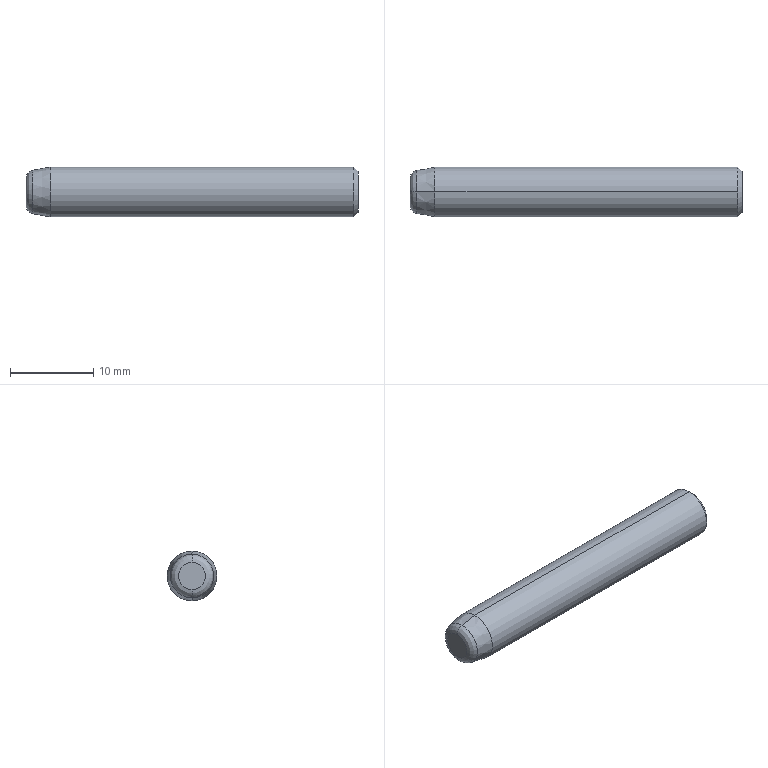Part | STEP file | Pino guia - PNG-0640 - M4 | 1 solid | 19 faces | box 40 x 6 x 6 mm | volume 979.582 mm3 | cone 8 | cylinder 6 | plane 3 | torus 2 | commonest cylinder face diameters 3.3 x2 4 x2 6 x2
STEP:
#1=CARTESIAN_POINT('',(0.,0.,0.));
#2=DIRECTION('',(0.,0.,1.));
#3=DIRECTION('',(1.,0.,0.));
#4=AXIS2_PLACEMENT_3D('',#1,#2,#3);
#5=CARTESIAN_POINT('',(-39.174,0.,2.617));
#6=VERTEX_POINT('',#5);
#7=CARTESIAN_POINT('',(-39.174,0.,-2.617));
#8=VERTEX_POINT('',#7);
#9=CARTESIAN_POINT('',(-39.174,0.,0.));
#10=DIRECTION('',(-1.,0.,0.));
#11=DIRECTION('',(0.,0.,1.));
#12=AXIS2_PLACEMENT_3D('',#9,#10,#11);
#13=CIRCLE('',#12,2.617);
#14=CARTESIAN_POINT('',(-39.,0.,0.));
#15=DIRECTION('',(-1.,0.,0.));
#16=DIRECTION('',(0.,0.,1.));
#17=AXIS2_PLACEMENT_3D('',#14,#15,#16);
#18=TOROIDAL_SURFACE('',#17,1.632,1.);
#19=CARTESIAN_POINT('',(0.,0.1745));
#20=DIRECTION('',(1.,0.));
#21=VECTOR('',#20,1.);
#22=LINE('',#19,#21);
#23=(GEOMETRIC_REPRESENTATION_CONTEXT(2)PARAMETRIC_REPRESENTATION_CONTEXT()REPRESENTATION_CONTEXT('',''));
#24=DEFINITIONAL_REPRESENTATION('',(#22),#23);
#25=PCURVE('',#18,#24);
#26=CARTESIAN_POINT('',(-37.,0.,0.));
#27=DIRECTION('',(1.,0.,0.));
#28=DIRECTION('',(0.,0.,-1.));
#29=AXIS2_PLACEMENT_3D('',#26,#27,#28);
#30=CONICAL_SURFACE('',#29,3.,0.1745);
#31=CARTESIAN_POINT('',(3.142,-2.174));
#32=DIRECTION('',(-1.,0.));
#33=VECTOR('',#32,1.);
#34=LINE('',#31,#33);
#35=(GEOMETRIC_REPRESENTATION_CONTEXT(2)PARAMETRIC_REPRESENTATION_CONTEXT()REPRESENTATION_CONTEXT('',''));
#36=DEFINITIONAL_REPRESENTATION('',(#34),#35);
#37=PCURVE('',#30,#36);
#38=SURFACE_CURVE('',#13,(#25,#37),.PCURVE_S1.);
#39=EDGE_CURVE('',#6,#8,#38,.T.);
#40=ORIENTED_EDGE('',*,*,#39,.T.);
#41=CARTESIAN_POINT('',(-40.,0.,-1.632));
#42=VERTEX_POINT('',#41);
#43=CARTESIAN_POINT('',(-39.,0.,-1.632));
#44=DIRECTION('',(0.,1.,0.));
#45=DIRECTION('',(0.,0.,1.));
#46=AXIS2_PLACEMENT_3D('',#43,#44,#45);
#47=CIRCLE('',#46,1.);
#48=CARTESIAN_POINT('',(3.142,-3.142));
#49=DIRECTION('',(0.,1.));
#50=VECTOR('',#49,1.);
#51=LINE('',#48,#50);
#52=(GEOMETRIC_REPRESENTATION_CONTEXT(2)PARAMETRIC_REPRESENTATION_CONTEXT()REPRESENTATION_CONTEXT('',''));
#53=DEFINITIONAL_REPRESENTATION('',(#51),#52);
#54=PCURVE('',#18,#53);
#55=CARTESIAN_POINT('',(-39.,0.,0.));
#56=DIRECTION('',(-1.,0.,0.));
#57=DIRECTION('',(0.,0.,1.));
#58=AXIS2_PLACEMENT_3D('',#55,#56,#57);
#59=TOROIDAL_SURFACE('',#58,1.632,1.);
#60=CARTESIAN_POINT('',(3.142,-3.142));
#61=DIRECTION('',(0.,1.));
#62=VECTOR('',#61,1.);
#63=LINE('',#60,#62);
#64=(GEOMETRIC_REPRESENTATION_CONTEXT(2)PARAMETRIC_REPRESENTATION_CONTEXT()REPRESENTATION_CONTEXT('',''));
#65=DEFINITIONAL_REPRESENTATION('',(#63),#64);
#66=PCURVE('',#59,#65);
#67=SURFACE_CURVE('',#47,(#54,#66),.PCURVE_S1.);
#68=EDGE_CURVE('',#8,#42,#67,.T.);
#69=ORIENTED_EDGE('',*,*,#68,.T.);
#70=CARTESIAN_POINT('',(-40.,0.,1.632));
#71=VERTEX_POINT('',#70);
#72=CARTESIAN_POINT('',(-40.,0.,0.));
#73=DIRECTION('',(-1.,0.,0.));
#74=DIRECTION('',(0.,0.,1.));
#75=AXIS2_PLACEMENT_3D('',#72,#73,#74);
#76=CIRCLE('',#75,1.632);
#77=CARTESIAN_POINT('',(0.,1.571));
#78=DIRECTION('',(1.,0.));
#79=VECTOR('',#78,1.);
#80=LINE('',#77,#79);
#81=(GEOMETRIC_REPRESENTATION_CONTEXT(2)PARAMETRIC_REPRESENTATION_CONTEXT()REPRESENTATION_CONTEXT('',''));
#82=DEFINITIONAL_REPRESENTATION('',(#80),#81);
#83=PCURVE('',#18,#82);
#84=CARTESIAN_POINT('',(-40.,0.,-1.632));
#85=DIRECTION('',(1.,0.,0.));
#86=DIRECTION('',(0.,0.,-1.));
#87=AXIS2_PLACEMENT_3D('',#84,#85,#86);
#88=PLANE('',#87);
#89=CARTESIAN_POINT('',(-3.264,0.));
#90=CARTESIAN_POINT('',(-3.264,2.827));
#91=CARTESIAN_POINT('',(-0.816,1.413));
#92=CARTESIAN_POINT('',(1.632,0.));
#93=CARTESIAN_POINT('',(-0.816,-1.413));
#94=CARTESIAN_POINT('',(-3.264,-2.827));
#95=CARTESIAN_POINT('',(-3.264,0.));
#96=(BOUNDED_CURVE()B_SPLINE_CURVE(2,(#89,#90,#91,#92,#93,#94,#95),.UNSPECIFIED.,.T.,.F.)B_SPLINE_CURVE_WITH_KNOTS((1,2,2,2,2,1),(-2.094,0.,2.094,4.189,6.283,8.378),.UNSPECIFIED.)CURVE()GEOMETRIC_REPRESENTATION_ITEM()RATIONAL_B_SPLINE_CURVE((1.,0.5,1.,0.5,1.,0.5,1.))REPRESENTATION_ITEM(''));
#97=(GEOMETRIC_REPRESENTATION_CONTEXT(2)PARAMETRIC_REPRESENTATION_CONTEXT()REPRESENTATION_CONTEXT('',''));
#98=DEFINITIONAL_REPRESENTATION('',(#96),#97);
#99=PCURVE('',#88,#98);
#100=SURFACE_CURVE('',#76,(#83,#99),.PCURVE_S1.);
#101=EDGE_CURVE('',#71,#42,#100,.T.);
#102=ORIENTED_EDGE('',*,*,#101,.F.);
#103=CARTESIAN_POINT('',(-39.,0.,1.632));
#104=DIRECTION('',(0.,-1.,0.));
#105=DIRECTION('',(0.,0.,-1.));
#106=AXIS2_PLACEMENT_3D('',#103,#104,#105);
#107=CIRCLE('',#106,1.);
#108=CARTESIAN_POINT('',(0.,-3.142));
#109=DIRECTION('',(0.,1.));
#110=VECTOR('',#109,1.);
#111=LINE('',#108,#110);
#112=(GEOMETRIC_REPRESENTATION_CONTEXT(2)PARAMETRIC_REPRESENTATION_CONTEXT()REPRESENTATION_CONTEXT('',''));
#113=DEFINITIONAL_REPRESENTATION('',(#111),#112);
#114=PCURVE('',#18,#113);
#115=CARTESIAN_POINT('',(6.283,-3.142));
#116=DIRECTION('',(0.,1.));
#117=VECTOR('',#116,1.);
#118=LINE('',#115,#117);
#119=(GEOMETRIC_REPRESENTATION_CONTEXT(2)PARAMETRIC_REPRESENTATION_CONTEXT()REPRESENTATION_CONTEXT('',''));
#120=DEFINITIONAL_REPRESENTATION('',(#118),#119);
#121=PCURVE('',#59,#120);
#122=SURFACE_CURVE('',#107,(#114,#121),.PCURVE_S1.);
#123=EDGE_CURVE('',#6,#71,#122,.T.);
#124=ORIENTED_EDGE('',*,*,#123,.F.);
#125=EDGE_LOOP('',(#40,#69,#102,#124));
#126=FACE_BOUND('',#125,.T.);
#127=ADVANCED_FACE('',(#126),#18,.T.);
#128=ORIENTED_EDGE('',*,*,#39,.F.);
#129=CARTESIAN_POINT('',(-37.,0.,3.));
#130=VERTEX_POINT('',#129);
#131=CARTESIAN_POINT('',(-37.,0.,3.));
#132=DIRECTION('',(0.9848,0.,0.1736));
#133=VECTOR('',#132,1.);
#134=LINE('',#131,#133);
#135=CARTESIAN_POINT('',(3.142,0.));
#136=DIRECTION('',(0.,1.));
#137=VECTOR('',#136,1.);
#138=LINE('',#135,#137);
#139=(GEOMETRIC_REPRESENTATION_CONTEXT(2)PARAMETRIC_REPRESENTATION_CONTEXT()REPRESENTATION_CONTEXT('',''));
#140=DEFINITIONAL_REPRESENTATION('',(#138),#139);
#141=PCURVE('',#30,#140);
#142=CARTESIAN_POINT('',(-37.,0.,0.));
#143=DIRECTION('',(1.,0.,0.));
#144=DIRECTION('',(0.,0.,-1.));
#145=AXIS2_PLACEMENT_3D('',#142,#143,#144);
#146=CONICAL_SURFACE('',#145,3.,0.1745);
#147=CARTESIAN_POINT('',(3.142,0.));
#148=DIRECTION('',(0.,1.));
#149=VECTOR('',#148,1.);
#150=LINE('',#147,#149);
#151=(GEOMETRIC_REPRESENTATION_CONTEXT(2)PARAMETRIC_REPRESENTATION_CONTEXT()REPRESENTATION_CONTEXT('',''));
#152=DEFINITIONAL_REPRESENTATION('',(#150),#151);
#153=PCURVE('',#146,#152);
#154=SURFACE_CURVE('',#134,(#141,#153),.PCURVE_S1.);
#155=EDGE_CURVE('',#6,#130,#154,.T.);
#156=ORIENTED_EDGE('',*,*,#155,.T.);
#157=CARTESIAN_POINT('',(-37.,0.,-3.));
#158=VERTEX_POINT('',#157);
#159=CARTESIAN_POINT('',(-37.,0.,0.));
#160=DIRECTION('',(-1.,0.,0.));
#161=DIRECTION('',(0.,0.,1.));
#162=AXIS2_PLACEMENT_3D('',#159,#160,#161);
#163=CIRCLE('',#162,3.);
#164=CARTESIAN_POINT('',(3.142,0.));
#165=DIRECTION('',(-1.,0.));
#166=VECTOR('',#165,1.);
#167=LINE('',#164,#166);
#168=(GEOMETRIC_REPRESENTATION_CONTEXT(2)PARAMETRIC_REPRESENTATION_CONTEXT()REPRESENTATION_CONTEXT('',''));
#169=DEFINITIONAL_REPRESENTATION('',(#167),#168);
#170=PCURVE('',#30,#169);
#171=CARTESIAN_POINT('',(-5.343,0.,0.));
#172=DIRECTION('',(-1.,0.,0.));
#173=DIRECTION('',(0.,0.,1.));
#174=AXIS2_PLACEMENT_3D('',#171,#172,#173);
#175=CYLINDRICAL_SURFACE('',#174,3.);
#176=CARTESIAN_POINT('',(0.,31.657));
#177=DIRECTION('',(1.,0.));
#178=VECTOR('',#177,1.);
#179=LINE('',#176,#178);
#180=(GEOMETRIC_REPRESENTATION_CONTEXT(2)PARAMETRIC_REPRESENTATION_CONTEXT()REPRESENTATION_CONTEXT('',''));
#181=DEFINITIONAL_REPRESENTATION('',(#179),#180);
#182=PCURVE('',#175,#181);
#183=SURFACE_CURVE('',#163,(#170,#182),.PCURVE_S1.);
#184=EDGE_CURVE('',#130,#158,#183,.T.);
#185=ORIENTED_EDGE('',*,*,#184,.T.);
#186=CARTESIAN_POINT('',(-37.,0.,-3.));
#187=DIRECTION('',(0.9848,0.,-0.1736));
#188=VECTOR('',#187,1.);
#189=LINE('',#186,#188);
#190=CARTESIAN_POINT('',(0.,0.));
#191=DIRECTION('',(0.,1.));
#192=VECTOR('',#191,1.);
#193=LINE('',#190,#192);
#194=(GEOMETRIC_REPRESENTATION_CONTEXT(2)PARAMETRIC_REPRESENTATION_CONTEXT()REPRESENTATION_CONTEXT('',''));
#195=DEFINITIONAL_REPRESENTATION('',(#193),#194);
#196=PCURVE('',#30,#195);
#197=CARTESIAN_POINT('',(6.283,0.));
#198=DIRECTION('',(0.,1.));
#199=VECTOR('',#198,1.);
#200=LINE('',#197,#199);
#201=(GEOMETRIC_REPRESENTATION_CONTEXT(2)PARAMETRIC_REPRESENTATION_CONTEXT()REPRESENTATION_CONTEXT('',''));
#202=DEFINITIONAL_REPRESENTATION('',(#200),#201);
#203=PCURVE('',#146,#202);
#204=SURFACE_CURVE('',#189,(#196,#203),.PCURVE_S1.);
#205=EDGE_CURVE('',#8,#158,#204,.T.);
#206=ORIENTED_EDGE('',*,*,#205,.F.);
#207=EDGE_LOOP('',(#128,#156,#185,#206));
#208=FACE_BOUND('',#207,.T.);
#209=ADVANCED_FACE('',(#208),#30,.T.);
#210=CARTESIAN_POINT('',(-0.025,0.,-2.));
#211=VERTEX_POINT('',#210);
#212=CARTESIAN_POINT('',(0.,0.,-2.025));
#213=VERTEX_POINT('',#212);
#214=CARTESIAN_POINT('',(0.,0.,-2.025));
#215=DIRECTION('',(0.7071,0.,-0.7071));
#216=VECTOR('',#215,1.);
#217=LINE('',#214,#216);
#218=CARTESIAN_POINT('',(0.,0.,0.));
#219=DIRECTION('',(1.,0.,0.));
#220=DIRECTION('',(0.,0.,-1.));
#221=AXIS2_PLACEMENT_3D('',#218,#219,#220);
#222=CONICAL_SURFACE('',#221,2.025,0.7854);
#223=CARTESIAN_POINT('',(6.283,0.));
#224=DIRECTION('',(0.,1.));
#225=VECTOR('',#224,1.);
#226=LINE('',#223,#225);
#227=(GEOMETRIC_REPRESENTATION_CONTEXT(2)PARAMETRIC_REPRESENTATION_CONTEXT()REPRESENTATION_CONTEXT('',''));
#228=DEFINITIONAL_REPRESENTATION('',(#226),#227);
#229=PCURVE('',#222,#228);
#230=CARTESIAN_POINT('',(0.,0.,0.));
#231=DIRECTION('',(1.,0.,0.));
#232=DIRECTION('',(0.,0.,-1.));
#233=AXIS2_PLACEMENT_3D('',#230,#231,#232);
#234=CONICAL_SURFACE('',#233,2.025,0.7854);
#235=CARTESIAN_POINT('',(0.,0.));
#236=DIRECTION('',(0.,1.));
#237=VECTOR('',#236,1.);
#238=LINE('',#235,#237);
#239=(GEOMETRIC_REPRESENTATION_CONTEXT(2)PARAMETRIC_REPRESENTATION_CONTEXT()REPRESENTATION_CONTEXT('',''));
#240=DEFINITIONAL_REPRESENTATION('',(#238),#239);
#241=PCURVE('',#234,#240);
#242=SURFACE_CURVE('',#217,(#229,#241),.PCURVE_S1.);
#243=EDGE_CURVE('',#211,#213,#242,.T.);
#244=ORIENTED_EDGE('',*,*,#243,.T.);
#245=CARTESIAN_POINT('',(0.,0.,2.025));
#246=VERTEX_POINT('',#245);
#247=CARTESIAN_POINT('',(0.,0.,0.));
#248=DIRECTION('',(1.,0.,0.));
#249=DIRECTION('',(0.,0.,-1.));
#250=AXIS2_PLACEMENT_3D('',#247,#248,#249);
#251=CIRCLE('',#250,2.025);
#252=CARTESIAN_POINT('',(0.,0.));
#253=DIRECTION('',(1.,0.));
#254=VECTOR('',#253,1.);
#255=LINE('',#252,#254);
#256=(GEOMETRIC_REPRESENTATION_CONTEXT(2)PARAMETRIC_REPRESENTATION_CONTEXT()REPRESENTATION_CONTEXT('',''));
#257=DEFINITIONAL_REPRESENTATION('',(#255),#256);
#258=PCURVE('',#222,#257);
#259=CARTESIAN_POINT('',(0.,2.5,0.));
#260=DIRECTION('',(-1.,0.,0.));
#261=DIRECTION('',(0.,0.,1.));
#262=AXIS2_PLACEMENT_3D('',#259,#260,#261);
#263=PLANE('',#262);
#264=CARTESIAN_POINT('',(-2.025,-2.5));
#265=CARTESIAN_POINT('',(-2.025,1.007));
#266=CARTESIAN_POINT('',(1.012,-0.7463));
#267=CARTESIAN_POINT('',(4.05,-2.5));
#268=CARTESIAN_POINT('',(1.012,-4.254));
#269=CARTESIAN_POINT('',(-2.025,-6.007));
#270=CARTESIAN_POINT('',(-2.025,-2.5));
#271=(BOUNDED_CURVE()B_SPLINE_CURVE(2,(#264,#265,#266,#267,#268,#269,#270),.UNSPECIFIED.,.T.,.F.)B_SPLINE_CURVE_WITH_KNOTS((1,2,2,2,2,1),(-2.094,0.,2.094,4.189,6.283,8.378),.UNSPECIFIED.)CURVE()GEOMETRIC_REPRESENTATION_ITEM()RATIONAL_B_SPLINE_CURVE((1.,0.5,1.,0.5,1.,0.5,1.))REPRESENTATION_ITEM(''));
#272=(GEOMETRIC_REPRESENTATION_CONTEXT(2)PARAMETRIC_REPRESENTATION_CONTEXT()REPRESENTATION_CONTEXT('',''));
#273=DEFINITIONAL_REPRESENTATION('',(#271),#272);
#274=PCURVE('',#263,#273);
#275=SURFACE_CURVE('',#251,(#258,#274),.PCURVE_S1.);
#276=EDGE_CURVE('',#246,#213,#275,.T.);
#277=ORIENTED_EDGE('',*,*,#276,.F.);
#278=CARTESIAN_POINT('',(-0.025,0.,2.));
#279=VERTEX_POINT('',#278);
#280=CARTESIAN_POINT('',(0.,0.,2.025));
#281=DIRECTION('',(0.7071,0.,0.7071));
#282=VECTOR('',#281,1.);
#283=LINE('',#280,#282);
#284=CARTESIAN_POINT('',(3.142,0.));
#285=DIRECTION('',(0.,1.));
#286=VECTOR('',#285,1.);
#287=LINE('',#284,#286);
#288=(GEOMETRIC_REPRESENTATION_CONTEXT(2)PARAMETRIC_REPRESENTATION_CONTEXT()REPRESENTATION_CONTEXT('',''));
#289=DEFINITIONAL_REPRESENTATION('',(#287),#288);
#290=PCURVE('',#222,#289);
#291=CARTESIAN_POINT('',(3.142,0.));
#292=DIRECTION('',(0.,1.));
#293=VECTOR('',#292,1.);
#294=LINE('',#291,#293);
#295=(GEOMETRIC_REPRESENTATION_CONTEXT(2)PARAMETRIC_REPRESENTATION_CONTEXT()REPRESENTATION_CONTEXT('',''));
#296=DEFINITIONAL_REPRESENTATION('',(#294),#295);
#297=PCURVE('',#234,#296);
#298=SURFACE_CURVE('',#283,(#290,#297),.PCURVE_S1.);
#299=EDGE_CURVE('',#279,#246,#298,.T.);
#300=ORIENTED_EDGE('',*,*,#299,.F.);
#301=CARTESIAN_POINT('',(-0.025,0.,0.));
#302=DIRECTION('',(1.,0.,0.));
#303=DIRECTION('',(0.,0.,-1.));
#304=AXIS2_PLACEMENT_3D('',#301,#302,#303);
#305=CIRCLE('',#304,2.);
#306=CARTESIAN_POINT('',(0.,-0.025));
#307=DIRECTION('',(1.,0.));
#308=VECTOR('',#307,1.);
#309=LINE('',#306,#308);
#310=(GEOMETRIC_REPRESENTATION_CONTEXT(2)PARAMETRIC_REPRESENTATION_CONTEXT()REPRESENTATION_CONTEXT('',''));
#311=DEFINITIONAL_REPRESENTATION('',(#309),#310);
#312=PCURVE('',#222,#311);
#313=CARTESIAN_POINT('',(0.,0.,0.));
#314=DIRECTION('',(1.,0.,0.));
#315=DIRECTION('',(0.,0.,-1.));
#316=AXIS2_PLACEMENT_3D('',#313,#314,#315);
#317=CYLINDRICAL_SURFACE('',#316,2.);
#318=CARTESIAN_POINT('',(0.,-0.025));
#319=DIRECTION('',(1.,0.));
#320=VECTOR('',#319,1.);
#321=LINE('',#318,#320);
#322=(GEOMETRIC_REPRESENTATION_CONTEXT(2)PARAMETRIC_REPRESENTATION_CONTEXT()REPRESENTATION_CONTEXT('',''));
#323=DEFINITIONAL_REPRESENTATION('',(#321),#322);
#324=PCURVE('',#317,#323);
#325=SURFACE_CURVE('',#305,(#312,#324),.PCURVE_S1.);
#326=EDGE_CURVE('',#279,#211,#325,.T.);
#327=ORIENTED_EDGE('',*,*,#326,.T.);
#328=EDGE_LOOP('',(#244,#277,#300,#327));
#329=FACE_BOUND('',#328,.F.);
#330=ADVANCED_FACE('',(#329),#222,.F.);
#331=CARTESIAN_POINT('',(-9.,0.,-2.));
#332=VERTEX_POINT('',#331);
#333=CARTESIAN_POINT('',(0.,0.,-2.));
#334=DIRECTION('',(1.,0.,0.));
#335=VECTOR('',#334,1.);
#336=LINE('',#333,#335);
#337=CARTESIAN_POINT('',(6.283,0.));
#338=DIRECTION('',(0.,1.));
#339=VECTOR('',#338,1.);
#340=LINE('',#337,#339);
#341=(GEOMETRIC_REPRESENTATION_CONTEXT(2)PARAMETRIC_REPRESENTATION_CONTEXT()REPRESENTATION_CONTEXT('',''));
#342=DEFINITIONAL_REPRESENTATION('',(#340),#341);
#343=PCURVE('',#317,#342);
#344=CARTESIAN_POINT('',(0.,0.,0.));
#345=DIRECTION('',(1.,0.,0.));
#346=DIRECTION('',(0.,0.,-1.));
#347=AXIS2_PLACEMENT_3D('',#344,#345,#346);
#348=CYLINDRICAL_SURFACE('',#347,2.);
#349=CARTESIAN_POINT('',(0.,0.));
#350=DIRECTION('',(0.,1.));
#351=VECTOR('',#350,1.);
#352=LINE('',#349,#351);
#353=(GEOMETRIC_REPRESENTATION_CONTEXT(2)PARAMETRIC_REPRESENTATION_CONTEXT()REPRESENTATION_CONTEXT('',''));
#354=DEFINITIONAL_REPRESENTATION('',(#352),#353);
#355=PCURVE('',#348,#354);
#356=SURFACE_CURVE('',#336,(#343,#355),.PCURVE_S1.);
#357=EDGE_CURVE('',#332,#211,#356,.T.);
#358=ORIENTED_EDGE('',*,*,#357,.T.);
#359=ORIENTED_EDGE('',*,*,#326,.F.);
#360=CARTESIAN_POINT('',(-9.,0.,2.));
#361=VERTEX_POINT('',#360);
#362=CARTESIAN_POINT('',(0.,0.,2.));
#363=DIRECTION('',(1.,0.,0.));
#364=VECTOR('',#363,1.);
#365=LINE('',#362,#364);
#366=CARTESIAN_POINT('',(3.142,0.));
#367=DIRECTION('',(0.,1.));
#368=VECTOR('',#367,1.);
#369=LINE('',#366,#368);
#370=(GEOMETRIC_REPRESENTATION_CONTEXT(2)PARAMETRIC_REPRESENTATION_CONTEXT()REPRESENTATION_CONTEXT('',''));
#371=DEFINITIONAL_REPRESENTATION('',(#369),#370);
#372=PCURVE('',#317,#371);
#373=CARTESIAN_POINT('',(3.142,0.));
#374=DIRECTION('',(0.,1.));
#375=VECTOR('',#374,1.);
#376=LINE('',#373,#375);
#377=(GEOMETRIC_REPRESENTATION_CONTEXT(2)PARAMETRIC_REPRESENTATION_CONTEXT()REPRESENTATION_CONTEXT('',''));
#378=DEFINITIONAL_REPRESENTATION('',(#376),#377);
#379=PCURVE('',#348,#378);
#380=SURFACE_CURVE('',#365,(#372,#379),.PCURVE_S1.);
#381=EDGE_CURVE('',#361,#279,#380,.T.);
#382=ORIENTED_EDGE('',*,*,#381,.F.);
#383=CARTESIAN_POINT('',(-9.,0.,0.));
#384=DIRECTION('',(1.,0.,0.));
#385=DIRECTION('',(0.,0.,-1.));
#386=AXIS2_PLACEMENT_3D('',#383,#384,#385);
#387=CIRCLE('',#386,2.);
#388=CARTESIAN_POINT('',(0.,-9.));
#389=DIRECTION('',(1.,0.));
#390=VECTOR('',#389,1.);
#391=LINE('',#388,#390);
#392=(GEOMETRIC_REPRESENTATION_CONTEXT(2)PARAMETRIC_REPRESENTATION_CONTEXT()REPRESENTATION_CONTEXT('',''));
#393=DEFINITIONAL_REPRESENTATION('',(#391),#392);
#394=PCURVE('',#317,#393);
#395=CARTESIAN_POINT('',(-9.,1.65,0.));
#396=DIRECTION('',(-1.,0.,0.));
#397=DIRECTION('',(0.,0.,1.));
#398=AXIS2_PLACEMENT_3D('',#395,#396,#397);
#399=PLANE('',#398);
#400=CARTESIAN_POINT('',(-2.,-1.65));
#401=CARTESIAN_POINT('',(-2.,1.814));
#402=CARTESIAN_POINT('',(1.,0.08205));
#403=CARTESIAN_POINT('',(4.,-1.65));
#404=CARTESIAN_POINT('',(1.,-3.382));
#405=CARTESIAN_POINT('',(-2.,-5.114));
#406=CARTESIAN_POINT('',(-2.,-1.65));
#407=(BOUNDED_CURVE()B_SPLINE_CURVE(2,(#400,#401,#402,#403,#404,#405,#406),.UNSPECIFIED.,.T.,.F.)B_SPLINE_CURVE_WITH_KNOTS((1,2,2,2,2,1),(-2.094,0.,2.094,4.189,6.283,8.378),.UNSPECIFIED.)CURVE()GEOMETRIC_REPRESENTATION_ITEM()RATIONAL_B_SPLINE_CURVE((1.,0.5,1.,0.5,1.,0.5,1.))REPRESENTATION_ITEM(''));
#408=(GEOMETRIC_REPRESENTATION_CONTEXT(2)PARAMETRIC_REPRESENTATION_CONTEXT()REPRESENTATION_CONTEXT('',''));
#409=DEFINITIONAL_REPRESENTATION('',(#407),#408);
#410=PCURVE('',#399,#409);
#411=SURFACE_CURVE('',#387,(#394,#410),.PCURVE_S1.);
#412=EDGE_CURVE('',#361,#332,#411,.T.);
#413=ORIENTED_EDGE('',*,*,#412,.T.);
#414=EDGE_LOOP('',(#358,#359,#382,#413));
#415=FACE_BOUND('',#414,.F.);
#416=ADVANCED_FACE('',(#415),#317,.F.);
#417=CARTESIAN_POINT('',(-11.,0.,-1.65));
#418=VERTEX_POINT('',#417);
#419=CARTESIAN_POINT('',(-9.,0.,-1.65));
#420=VERTEX_POINT('',#419);
#421=CARTESIAN_POINT('',(0.,0.,-1.65));
#422=DIRECTION('',(1.,0.,0.));
#423=VECTOR('',#422,1.);
#424=LINE('',#421,#423);
#425=CARTESIAN_POINT('',(0.,0.,0.));
#426=DIRECTION('',(1.,0.,0.));
#427=DIRECTION('',(0.,0.,-1.));
#428=AXIS2_PLACEMENT_3D('',#425,#426,#427);
#429=CYLINDRICAL_SURFACE('',#428,1.65);
#430=CARTESIAN_POINT('',(6.283,0.));
#431=DIRECTION('',(0.,1.));
#432=VECTOR('',#431,1.);
#433=LINE('',#430,#432);
#434=(GEOMETRIC_REPRESENTATION_CONTEXT(2)PARAMETRIC_REPRESENTATION_CONTEXT()REPRESENTATION_CONTEXT('',''));
#435=DEFINITIONAL_REPRESENTATION('',(#433),#434);
#436=PCURVE('',#429,#435);
#437=CARTESIAN_POINT('',(0.,0.,0.));
#438=DIRECTION('',(1.,0.,0.));
#439=DIRECTION('',(0.,0.,-1.));
#440=AXIS2_PLACEMENT_3D('',#437,#438,#439);
#441=CYLINDRICAL_SURFACE('',#440,1.65);
#442=CARTESIAN_POINT('',(0.,0.));
#443=DIRECTION('',(0.,1.));
#444=VECTOR('',#443,1.);
#445=LINE('',#442,#444);
#446=(GEOMETRIC_REPRESENTATION_CONTEXT(2)PARAMETRIC_REPRESENTATION_CONTEXT()REPRESENTATION_CONTEXT('',''));
#447=DEFINITIONAL_REPRESENTATION('',(#445),#446);
#448=PCURVE('',#441,#447);
#449=SURFACE_CURVE('',#424,(#436,#448),.PCURVE_S1.);
#450=EDGE_CURVE('',#418,#420,#449,.T.);
#451=ORIENTED_EDGE('',*,*,#450,.T.);
#452=CARTESIAN_POINT('',(-9.,0.,1.65));
#453=VERTEX_POINT('',#452);
#454=CARTESIAN_POINT('',(-9.,0.,0.));
#455=DIRECTION('',(1.,0.,0.));
#456=DIRECTION('',(0.,0.,-1.));
#457=AXIS2_PLACEMENT_3D('',#454,#455,#456);
#458=CIRCLE('',#457,1.65);
#459=CARTESIAN_POINT('',(0.,-9.));
#460=DIRECTION('',(1.,0.));
#461=VECTOR('',#460,1.);
#462=LINE('',#459,#461);
#463=(GEOMETRIC_REPRESENTATION_CONTEXT(2)PARAMETRIC_REPRESENTATION_CONTEXT()REPRESENTATION_CONTEXT('',''));
#464=DEFINITIONAL_REPRESENTATION('',(#462),#463);
#465=PCURVE('',#429,#464);
#466=CARTESIAN_POINT('',(-1.65,-1.65));
#467=CARTESIAN_POINT('',(-1.65,1.208));
#468=CARTESIAN_POINT('',(0.825,-0.2211));
#469=CARTESIAN_POINT('',(3.3,-1.65));
#470=CARTESIAN_POINT('',(0.825,-3.079));
#471=CARTESIAN_POINT('',(-1.65,-4.508));
#472=CARTESIAN_POINT('',(-1.65,-1.65));
#473=(BOUNDED_CURVE()B_SPLINE_CURVE(2,(#466,#467,#468,#469,#470,#471,#472),.UNSPECIFIED.,.T.,.F.)B_SPLINE_CURVE_WITH_KNOTS((1,2,2,2,2,1),(-2.094,0.,2.094,4.189,6.283,8.378),.UNSPECIFIED.)CURVE()GEOMETRIC_REPRESENTATION_ITEM()RATIONAL_B_SPLINE_CURVE((1.,0.5,1.,0.5,1.,0.5,1.))REPRESENTATION_ITEM(''));
#474=(GEOMETRIC_REPRESENTATION_CONTEXT(2)PARAMETRIC_REPRESENTATION_CONTEXT()REPRESENTATION_CONTEXT('',''));
#475=DEFINITIONAL_REPRESENTATION('',(#473),#474);
#476=PCURVE('',#399,#475);
#477=SURFACE_CURVE('',#458,(#465,#476),.PCURVE_S1.);
#478=EDGE_CURVE('',#453,#420,#477,.T.);
#479=ORIENTED_EDGE('',*,*,#478,.F.);
#480=CARTESIAN_POINT('',(-11.,0.,1.65));
#481=VERTEX_POINT('',#480);
#482=CARTESIAN_POINT('',(0.,0.,1.65));
#483=DIRECTION('',(1.,0.,0.));
#484=VECTOR('',#483,1.);
#485=LINE('',#482,#484);
#486=CARTESIAN_POINT('',(3.142,0.));
#487=DIRECTION('',(0.,1.));
#488=VECTOR('',#487,1.);
#489=LINE('',#486,#488);
#490=(GEOMETRIC_REPRESENTATION_CONTEXT(2)PARAMETRIC_REPRESENTATION_CONTEXT()REPRESENTATION_CONTEXT('',''));
#491=DEFINITIONAL_REPRESENTATION('',(#489),#490);
#492=PCURVE('',#429,#491);
#493=CARTESIAN_POINT('',(3.142,0.));
#494=DIRECTION('',(0.,1.));
#495=VECTOR('',#494,1.);
#496=LINE('',#493,#495);
#497=(GEOMETRIC_REPRESENTATION_CONTEXT(2)PARAMETRIC_REPRESENTATION_CONTEXT()REPRESENTATION_CONTEXT('',''));
#498=DEFINITIONAL_REPRESENTATION('',(#496),#497);
#499=PCURVE('',#441,#498);
#500=SURFACE_CURVE('',#485,(#492,#499),.PCURVE_S1.);
#501=EDGE_CURVE('',#481,#453,#500,.T.);
#502=ORIENTED_EDGE('',*,*,#501,.F.);
#503=CARTESIAN_POINT('',(-11.,0.,0.));
#504=DIRECTION('',(1.,0.,0.));
#505=DIRECTION('',(0.,0.,-1.));
#506=AXIS2_PLACEMENT_3D('',#503,#504,#505);
#507=CIRCLE('',#506,1.65);
#508=CARTESIAN_POINT('',(0.,-11.));
#509=DIRECTION('',(1.,0.));
#510=VECTOR('',#509,1.);
#511=LINE('',#508,#510);
#512=(GEOMETRIC_REPRESENTATION_CONTEXT(2)PARAMETRIC_REPRESENTATION_CONTEXT()REPRESENTATION_CONTEXT('',''));
#513=DEFINITIONAL_REPRESENTATION('',(#511),#512);
#514=PCURVE('',#429,#513);
#515=CARTESIAN_POINT('',(-11.,0.,0.));
#516=DIRECTION('',(1.,0.,0.));
#517=DIRECTION('',(0.,0.,-1.));
#518=AXIS2_PLACEMENT_3D('',#515,#516,#517);
#519=CONICAL_SURFACE('',#518,1.65,1.03);
#520=CARTESIAN_POINT('',(0.,0.));
#521=DIRECTION('',(1.,0.));
#522=VECTOR('',#521,1.);
#523=LINE('',#520,#522);
#524=(GEOMETRIC_REPRESENTATION_CONTEXT(2)PARAMETRIC_REPRESENTATION_CONTEXT()REPRESENTATION_CONTEXT('',''));
#525=DEFINITIONAL_REPRESENTATION('',(#523),#524);
#526=PCURVE('',#519,#525);
#527=SURFACE_CURVE('',#507,(#514,#526),.PCURVE_S1.);
#528=EDGE_CURVE('',#481,#418,#527,.T.);
#529=ORIENTED_EDGE('',*,*,#528,.T.);
#530=EDGE_LOOP('',(#451,#479,#502,#529));
#531=FACE_BOUND('',#530,.F.);
#532=ADVANCED_FACE('',(#531),#429,.F.);
#533=ORIENTED_EDGE('',*,*,#528,.F.);
#534=CARTESIAN_POINT('',(-11.991,0.,0.));
#535=VERTEX_POINT('',#534);
#536=CARTESIAN_POINT('',(-11.,0.,1.65));
#537=DIRECTION('',(0.515,0.,0.8572));
#538=VECTOR('',#537,1.);
#539=LINE('',#536,#538);
#540=CARTESIAN_POINT('',(3.142,0.));
#541=DIRECTION('',(0.,1.));
#542=VECTOR('',#541,1.);
#543=LINE('',#540,#542);
#544=(GEOMETRIC_REPRESENTATION_CONTEXT(2)PARAMETRIC_REPRESENTATION_CONTEXT()REPRESENTATION_CONTEXT('',''));
#545=DEFINITIONAL_REPRESENTATION('',(#543),#544);
#546=PCURVE('',#519,#545);
#547=CARTESIAN_POINT('',(-11.,0.,0.));
#548=DIRECTION('',(1.,0.,0.));
#549=DIRECTION('',(0.,0.,-1.));
#550=AXIS2_PLACEMENT_3D('',#547,#548,#549);
#551=CONICAL_SURFACE('',#550,1.65,1.03);
#552=CARTESIAN_POINT('',(3.142,0.));
#553=DIRECTION('',(0.,1.));
#554=VECTOR('',#553,1.);
#555=LINE('',#552,#554);
#556=(GEOMETRIC_REPRESENTATION_CONTEXT(2)PARAMETRIC_REPRESENTATION_CONTEXT()REPRESENTATION_CONTEXT('',''));
#557=DEFINITIONAL_REPRESENTATION('',(#555),#556);
#558=PCURVE('',#551,#557);
#559=SURFACE_CURVE('',#539,(#546,#558),.PCURVE_S1.);
#560=EDGE_CURVE('',#535,#481,#559,.T.);
#561=ORIENTED_EDGE('',*,*,#560,.F.);
#562=CARTESIAN_POINT('',(-11.,0.,-1.65));
#563=DIRECTION('',(0.515,0.,-0.8572));
#564=VECTOR('',#563,1.);
#565=LINE('',#562,#564);
#566=CARTESIAN_POINT('',(6.283,0.));
#567=DIRECTION('',(0.,1.));
#568=VECTOR('',#567,1.);
#569=LINE('',#566,#568);
#570=(GEOMETRIC_REPRESENTATION_CONTEXT(2)PARAMETRIC_REPRESENTATION_CONTEXT()REPRESENTATION_CONTEXT('',''));
#571=DEFINITIONAL_REPRESENTATION('',(#569),#570);
#572=PCURVE('',#519,#571);
#573=CARTESIAN_POINT('',(0.,0.));
#574=DIRECTION('',(0.,1.));
#575=VECTOR('',#574,1.);
#576=LINE('',#573,#575);
#577=(GEOMETRIC_REPRESENTATION_CONTEXT(2)PARAMETRIC_REPRESENTATION_CONTEXT()REPRESENTATION_CONTEXT('',''));
#578=DEFINITIONAL_REPRESENTATION('',(#576),#577);
#579=PCURVE('',#551,#578);
#580=SURFACE_CURVE('',#565,(#572,#579),.PCURVE_S1.);
#581=EDGE_CURVE('',#535,#418,#580,.T.);
#582=ORIENTED_EDGE('',*,*,#581,.T.);
#583=EDGE_LOOP('',(#533,#561,#582));
#584=FACE_BOUND('',#583,.F.);
#585=ADVANCED_FACE('',(#584),#519,.F.);
#586=CARTESIAN_POINT('',(-0.5,0.,3.));
#587=VERTEX_POINT('',#586);
#588=CARTESIAN_POINT('',(-0.5,0.,-3.));
#589=VERTEX_POINT('',#588);
#590=CARTESIAN_POINT('',(-0.5,0.,0.));
#591=DIRECTION('',(-1.,0.,0.));
#592=DIRECTION('',(0.,0.,1.));
#593=AXIS2_PLACEMENT_3D('',#590,#591,#592);
#594=CIRCLE('',#593,3.);
#595=CARTESIAN_POINT('',(0.,-4.843));
#596=DIRECTION('',(1.,0.));
#597=VECTOR('',#596,1.);
#598=LINE('',#595,#597);
#599=(GEOMETRIC_REPRESENTATION_CONTEXT(2)PARAMETRIC_REPRESENTATION_CONTEXT()REPRESENTATION_CONTEXT('',''));
#600=DEFINITIONAL_REPRESENTATION('',(#598),#599);
#601=PCURVE('',#175,#600);
#602=CARTESIAN_POINT('',(0.,0.,0.));
#603=DIRECTION('',(-1.,0.,0.));
#604=DIRECTION('',(0.,0.,1.));
#605=AXIS2_PLACEMENT_3D('',#602,#603,#604);
#606=CONICAL_SURFACE('',#605,2.5,0.7854);
#607=CARTESIAN_POINT('',(0.,0.5));
#608=DIRECTION('',(1.,0.));
#609=VECTOR('',#608,1.);
#610=LINE('',#607,#609);
#611=(GEOMETRIC_REPRESENTATION_CONTEXT(2)PARAMETRIC_REPRESENTATION_CONTEXT()REPRESENTATION_CONTEXT('',''));
#612=DEFINITIONAL_REPRESENTATION('',(#610),#611);
#613=PCURVE('',#606,#612);
#614=SURFACE_CURVE('',#594,(#601,#613),.PCURVE_S1.);
#615=EDGE_CURVE('',#587,#589,#614,.T.);
#616=ORIENTED_EDGE('',*,*,#615,.T.);
#617=CARTESIAN_POINT('',(-5.343,0.,-3.));
#618=DIRECTION('',(-1.,0.,0.));
#619=VECTOR('',#618,1.);
#620=LINE('',#617,#619);
#621=CARTESIAN_POINT('',(3.142,0.));
#622=DIRECTION('',(0.,1.));
#623=VECTOR('',#622,1.);
#624=LINE('',#621,#623);
#625=(GEOMETRIC_REPRESENTATION_CONTEXT(2)PARAMETRIC_REPRESENTATION_CONTEXT()REPRESENTATION_CONTEXT('',''));
#626=DEFINITIONAL_REPRESENTATION('',(#624),#625);
#627=PCURVE('',#175,#626);
#628=CARTESIAN_POINT('',(-5.343,0.,0.));
#629=DIRECTION('',(-1.,0.,0.));
#630=DIRECTION('',(0.,0.,1.));
#631=AXIS2_PLACEMENT_3D('',#628,#629,#630);
#632=CYLINDRICAL_SURFACE('',#631,3.);
#633=CARTESIAN_POINT('',(3.142,0.));
#634=DIRECTION('',(0.,1.));
#635=VECTOR('',#634,1.);
#636=LINE('',#633,#635);
#637=(GEOMETRIC_REPRESENTATION_CONTEXT(2)PARAMETRIC_REPRESENTATION_CONTEXT()REPRESENTATION_CONTEXT('',''));
#638=DEFINITIONAL_REPRESENTATION('',(#636),#637);
#639=PCURVE('',#632,#638);
#640=SURFACE_CURVE('',#620,(#627,#639),.PCURVE_S1.);
#641=EDGE_CURVE('',#589,#158,#640,.T.);
#642=ORIENTED_EDGE('',*,*,#641,.T.);
#643=ORIENTED_EDGE('',*,*,#184,.F.);
#644=CARTESIAN_POINT('',(-5.343,0.,3.));
#645=DIRECTION('',(-1.,0.,0.));
#646=VECTOR('',#645,1.);
#647=LINE('',#644,#646);
#648=CARTESIAN_POINT('',(0.,0.));
#649=DIRECTION('',(0.,1.));
#650=VECTOR('',#649,1.);
#651=LINE('',#648,#650);
#652=(GEOMETRIC_REPRESENTATION_CONTEXT(2)PARAMETRIC_REPRESENTATION_CONTEXT()REPRESENTATION_CONTEXT('',''));
#653=DEFINITIONAL_REPRESENTATION('',(#651),#652);
#654=PCURVE('',#175,#653);
#655=CARTESIAN_POINT('',(6.283,0.));
#656=DIRECTION('',(0.,1.));
#657=VECTOR('',#656,1.);
#658=LINE('',#655,#657);
#659=(GEOMETRIC_REPRESENTATION_CONTEXT(2)PARAMETRIC_REPRESENTATION_CONTEXT()REPRESENTATION_CONTEXT('',''));
#660=DEFINITIONAL_REPRESENTATION('',(#658),#659);
#661=PCURVE('',#632,#660);
#662=SURFACE_CURVE('',#647,(#654,#661),.PCURVE_S1.);
#663=EDGE_CURVE('',#587,#130,#662,.T.);
#664=ORIENTED_EDGE('',*,*,#663,.F.);
#665=EDGE_LOOP('',(#616,#642,#643,#664));
#666=FACE_BOUND('',#665,.T.);
#667=ADVANCED_FACE('',(#666),#175,.T.);
#668=CARTESIAN_POINT('',(0.,0.,2.5));
#669=VERTEX_POINT('',#668);
#670=CARTESIAN_POINT('',(0.,0.,-2.5));
#671=VERTEX_POINT('',#670);
#672=CARTESIAN_POINT('',(0.,0.,0.));
#673=DIRECTION('',(-1.,0.,0.));
#674=DIRECTION('',(0.,0.,1.));
#675=AXIS2_PLACEMENT_3D('',#672,#673,#674);
#676=CIRCLE('',#675,2.5);
#677=CARTESIAN_POINT('',(0.,0.));
#678=DIRECTION('',(1.,0.));
#679=VECTOR('',#678,1.);
#680=LINE('',#677,#679);
#681=(GEOMETRIC_REPRESENTATION_CONTEXT(2)PARAMETRIC_REPRESENTATION_CONTEXT()REPRESENTATION_CONTEXT('',''));
#682=DEFINITIONAL_REPRESENTATION('',(#680),#681);
#683=PCURVE('',#606,#682);
#684=CARTESIAN_POINT('',(0.,-2.5));
#685=DIRECTION('',(1.,0.));
#686=AXIS2_PLACEMENT_2D('',#684,#685);
#687=CIRCLE('',#686,2.5);
#688=(GEOMETRIC_REPRESENTATION_CONTEXT(2)PARAMETRIC_REPRESENTATION_CONTEXT()REPRESENTATION_CONTEXT('',''));
#689=DEFINITIONAL_REPRESENTATION('',(#687),#688);
#690=PCURVE('',#263,#689);
#691=SURFACE_CURVE('',#676,(#683,#690),.PCURVE_S1.);
#692=EDGE_CURVE('',#669,#671,#691,.T.);
#693=ORIENTED_EDGE('',*,*,#692,.T.);
#694=CARTESIAN_POINT('',(0.,0.,-2.5));
#695=DIRECTION('',(-0.7071,0.,-0.7071));
#696=VECTOR('',#695,1.);
#697=LINE('',#694,#696);
#698=CARTESIAN_POINT('',(3.142,0.));
#699=DIRECTION('',(0.,1.));
#700=VECTOR('',#699,1.);
#701=LINE('',#698,#700);
#702=(GEOMETRIC_REPRESENTATION_CONTEXT(2)PARAMETRIC_REPRESENTATION_CONTEXT()REPRESENTATION_CONTEXT('',''));
#703=DEFINITIONAL_REPRESENTATION('',(#701),#702);
#704=PCURVE('',#606,#703);
#705=CARTESIAN_POINT('',(0.,0.,0.));
#706=DIRECTION('',(-1.,0.,0.));
#707=DIRECTION('',(0.,0.,1.));
#708=AXIS2_PLACEMENT_3D('',#705,#706,#707);
#709=CONICAL_SURFACE('',#708,2.5,0.7854);
#710=CARTESIAN_POINT('',(3.142,0.));
#711=DIRECTION('',(0.,1.));
#712=VECTOR('',#711,1.);
#713=LINE('',#710,#712);
#714=(GEOMETRIC_REPRESENTATION_CONTEXT(2)PARAMETRIC_REPRESENTATION_CONTEXT()REPRESENTATION_CONTEXT('',''));
#715=DEFINITIONAL_REPRESENTATION('',(#713),#714);
#716=PCURVE('',#709,#715);
#717=SURFACE_CURVE('',#697,(#704,#716),.PCURVE_S1.);
#718=EDGE_CURVE('',#671,#589,#717,.T.);
#719=ORIENTED_EDGE('',*,*,#718,.T.);
#720=ORIENTED_EDGE('',*,*,#615,.F.);
#721=CARTESIAN_POINT('',(0.,0.,2.5));
#722=DIRECTION('',(-0.7071,0.,0.7071));
#723=VECTOR('',#722,1.);
#724=LINE('',#721,#723);
#725=CARTESIAN_POINT('',(0.,0.));
#726=DIRECTION('',(0.,1.));
#727=VECTOR('',#726,1.);
#728=LINE('',#725,#727);
#729=(GEOMETRIC_REPRESENTATION_CONTEXT(2)PARAMETRIC_REPRESENTATION_CONTEXT()REPRESENTATION_CONTEXT('',''));
#730=DEFINITIONAL_REPRESENTATION('',(#728),#729);
#731=PCURVE('',#606,#730);
#732=CARTESIAN_POINT('',(6.283,0.));
#733=DIRECTION('',(0.,1.));
#734=VECTOR('',#733,1.);
#735=LINE('',#732,#734);
#736=(GEOMETRIC_REPRESENTATION_CONTEXT(2)PARAMETRIC_REPRESENTATION_CONTEXT()REPRESENTATION_CONTEXT('',''));
#737=DEFINITIONAL_REPRESENTATION('',(#735),#736);
#738=PCURVE('',#709,#737);
#739=SURFACE_CURVE('',#724,(#731,#738),.PCURVE_S1.);
#740=EDGE_CURVE('',#669,#587,#739,.T.);
#741=ORIENTED_EDGE('',*,*,#740,.F.);
#742=EDGE_LOOP('',(#693,#719,#720,#741));
#743=FACE_BOUND('',#742,.T.);
#744=ADVANCED_FACE('',(#743),#606,.T.);
#745=CARTESIAN_POINT('',(0.,0.,0.));
#746=DIRECTION('',(1.,0.,0.));
#747=DIRECTION('',(0.,0.,-1.));
#748=AXIS2_PLACEMENT_3D('',#745,#746,#747);
#749=CIRCLE('',#748,2.025);
#750=CARTESIAN_POINT('',(-2.025,-2.5));
#751=CARTESIAN_POINT('',(-2.025,1.007));
#752=CARTESIAN_POINT('',(1.012,-0.7463));
#753=CARTESIAN_POINT('',(4.05,-2.5));
#754=CARTESIAN_POINT('',(1.012,-4.254));
#755=CARTESIAN_POINT('',(-2.025,-6.007));
#756=CARTESIAN_POINT('',(-2.025,-2.5));
#757=(BOUNDED_CURVE()B_SPLINE_CURVE(2,(#750,#751,#752,#753,#754,#755,#756),.UNSPECIFIED.,.T.,.F.)B_SPLINE_CURVE_WITH_KNOTS((1,2,2,2,2,1),(-2.094,0.,2.094,4.189,6.283,8.378),.UNSPECIFIED.)CURVE()GEOMETRIC_REPRESENTATION_ITEM()RATIONAL_B_SPLINE_CURVE((1.,0.5,1.,0.5,1.,0.5,1.))REPRESENTATION_ITEM(''));
#758=(GEOMETRIC_REPRESENTATION_CONTEXT(2)PARAMETRIC_REPRESENTATION_CONTEXT()REPRESENTATION_CONTEXT('',''));
#759=DEFINITIONAL_REPRESENTATION('',(#757),#758);
#760=PCURVE('',#263,#759);
#761=CARTESIAN_POINT('',(0.,0.));
#762=DIRECTION('',(1.,0.));
#763=VECTOR('',#762,1.);
#764=LINE('',#761,#763);
#765=(GEOMETRIC_REPRESENTATION_CONTEXT(2)PARAMETRIC_REPRESENTATION_CONTEXT()REPRESENTATION_CONTEXT('',''));
#766=DEFINITIONAL_REPRESENTATION('',(#764),#765);
#767=PCURVE('',#234,#766);
#768=SURFACE_CURVE('',#749,(#760,#767),.PCURVE_S1.);
#769=EDGE_CURVE('',#213,#246,#768,.T.);
#770=ORIENTED_EDGE('',*,*,#769,.F.);
#771=ORIENTED_EDGE('',*,*,#276,.F.);
#772=EDGE_LOOP('',(#770,#771));
#773=FACE_BOUND('',#772,.T.);
#774=ORIENTED_EDGE('',*,*,#692,.F.);
#775=CARTESIAN_POINT('',(0.,0.,0.));
#776=DIRECTION('',(-1.,0.,0.));
#777=DIRECTION('',(0.,0.,1.));
#778=AXIS2_PLACEMENT_3D('',#775,#776,#777);
#779=CIRCLE('',#778,2.5);
#780=CARTESIAN_POINT('',(0.,-2.5));
#781=DIRECTION('',(1.,0.));
#782=AXIS2_PLACEMENT_2D('',#780,#781);
#783=CIRCLE('',#782,2.5);
#784=(GEOMETRIC_REPRESENTATION_CONTEXT(2)PARAMETRIC_REPRESENTATION_CONTEXT()REPRESENTATION_CONTEXT('',''));
#785=DEFINITIONAL_REPRESENTATION('',(#783),#784);
#786=PCURVE('',#263,#785);
#787=CARTESIAN_POINT('',(0.,0.));
#788=DIRECTION('',(1.,0.));
#789=VECTOR('',#788,1.);
#790=LINE('',#787,#789);
#791=(GEOMETRIC_REPRESENTATION_CONTEXT(2)PARAMETRIC_REPRESENTATION_CONTEXT()REPRESENTATION_CONTEXT('',''));
#792=DEFINITIONAL_REPRESENTATION('',(#790),#791);
#793=PCURVE('',#709,#792);
#794=SURFACE_CURVE('',#779,(#786,#793),.PCURVE_S1.);
#795=EDGE_CURVE('',#671,#669,#794,.T.);
#796=ORIENTED_EDGE('',*,*,#795,.F.);
#797=EDGE_LOOP('',(#774,#796));
#798=FACE_BOUND('',#797,.T.);
#799=ADVANCED_FACE('',(#773,#798),#263,.F.);
#800=ORIENTED_EDGE('',*,*,#718,.F.);
#801=ORIENTED_EDGE('',*,*,#795,.T.);
#802=ORIENTED_EDGE('',*,*,#740,.T.);
#803=CARTESIAN_POINT('',(-0.5,0.,0.));
#804=DIRECTION('',(-1.,0.,0.));
#805=DIRECTION('',(0.,0.,1.));
#806=AXIS2_PLACEMENT_3D('',#803,#804,#805);
#807=CIRCLE('',#806,3.);
#808=CARTESIAN_POINT('',(0.,0.5));
#809=DIRECTION('',(1.,0.));
#810=VECTOR('',#809,1.);
#811=LINE('',#808,#810);
#812=(GEOMETRIC_REPRESENTATION_CONTEXT(2)PARAMETRIC_REPRESENTATION_CONTEXT()REPRESENTATION_CONTEXT('',''));
#813=DEFINITIONAL_REPRESENTATION('',(#811),#812);
#814=PCURVE('',#709,#813);
#815=CARTESIAN_POINT('',(0.,-4.843));
#816=DIRECTION('',(1.,0.));
#817=VECTOR('',#816,1.);
#818=LINE('',#815,#817);
#819=(GEOMETRIC_REPRESENTATION_CONTEXT(2)PARAMETRIC_REPRESENTATION_CONTEXT()REPRESENTATION_CONTEXT('',''));
#820=DEFINITIONAL_REPRESENTATION('',(#818),#819);
#821=PCURVE('',#632,#820);
#822=SURFACE_CURVE('',#807,(#814,#821),.PCURVE_S1.);
#823=EDGE_CURVE('',#589,#587,#822,.T.);
#824=ORIENTED_EDGE('',*,*,#823,.F.);
#825=EDGE_LOOP('',(#800,#801,#802,#824));
#826=FACE_BOUND('',#825,.T.);
#827=ADVANCED_FACE('',(#826),#709,.T.);
#828=ORIENTED_EDGE('',*,*,#641,.F.);
#829=ORIENTED_EDGE('',*,*,#823,.T.);
#830=ORIENTED_EDGE('',*,*,#663,.T.);
#831=CARTESIAN_POINT('',(-37.,0.,0.));
#832=DIRECTION('',(-1.,0.,0.));
#833=DIRECTION('',(0.,0.,1.));
#834=AXIS2_PLACEMENT_3D('',#831,#832,#833);
#835=CIRCLE('',#834,3.);
#836=CARTESIAN_POINT('',(0.,31.657));
#837=DIRECTION('',(1.,0.));
#838=VECTOR('',#837,1.);
#839=LINE('',#836,#838);
#840=(GEOMETRIC_REPRESENTATION_CONTEXT(2)PARAMETRIC_REPRESENTATION_CONTEXT()REPRESENTATION_CONTEXT('',''));
#841=DEFINITIONAL_REPRESENTATION('',(#839),#840);
#842=PCURVE('',#632,#841);
#843=CARTESIAN_POINT('',(9.425,0.));
#844=DIRECTION('',(-1.,0.));
#845=VECTOR('',#844,1.);
#846=LINE('',#843,#845);
#847=(GEOMETRIC_REPRESENTATION_CONTEXT(2)PARAMETRIC_REPRESENTATION_CONTEXT()REPRESENTATION_CONTEXT('',''));
#848=DEFINITIONAL_REPRESENTATION('',(#846),#847);
#849=PCURVE('',#146,#848);
#850=SURFACE_CURVE('',#835,(#842,#849),.PCURVE_S1.);
#851=EDGE_CURVE('',#158,#130,#850,.T.);
#852=ORIENTED_EDGE('',*,*,#851,.F.);
#853=EDGE_LOOP('',(#828,#829,#830,#852));
#854=FACE_BOUND('',#853,.T.);
#855=ADVANCED_FACE('',(#854),#632,.T.);
#856=CARTESIAN_POINT('',(-11.,0.,0.));
#857=DIRECTION('',(1.,0.,0.));
#858=DIRECTION('',(0.,0.,-1.));
#859=AXIS2_PLACEMENT_3D('',#856,#857,#858);
#860=CIRCLE('',#859,1.65);
#861=CARTESIAN_POINT('',(0.,0.));
#862=DIRECTION('',(1.,0.));
#863=VECTOR('',#862,1.);
#864=LINE('',#861,#863);
#865=(GEOMETRIC_REPRESENTATION_CONTEXT(2)PARAMETRIC_REPRESENTATION_CONTEXT()REPRESENTATION_CONTEXT('',''));
#866=DEFINITIONAL_REPRESENTATION('',(#864),#865);
#867=PCURVE('',#551,#866);
#868=CARTESIAN_POINT('',(0.,-11.));
#869=DIRECTION('',(1.,0.));
#870=VECTOR('',#869,1.);
#871=LINE('',#868,#870);
#872=(GEOMETRIC_REPRESENTATION_CONTEXT(2)PARAMETRIC_REPRESENTATION_CONTEXT()REPRESENTATION_CONTEXT('',''));
#873=DEFINITIONAL_REPRESENTATION('',(#871),#872);
#874=PCURVE('',#441,#873);
#875=SURFACE_CURVE('',#860,(#867,#874),.PCURVE_S1.);
#876=EDGE_CURVE('',#418,#481,#875,.T.);
#877=ORIENTED_EDGE('',*,*,#876,.F.);
#878=ORIENTED_EDGE('',*,*,#581,.F.);
#879=ORIENTED_EDGE('',*,*,#560,.T.);
#880=EDGE_LOOP('',(#877,#878,#879));
#881=FACE_BOUND('',#880,.F.);
#882=ADVANCED_FACE('',(#881),#551,.F.);
#883=CARTESIAN_POINT('',(-9.,0.,0.));
#884=DIRECTION('',(1.,0.,0.));
#885=DIRECTION('',(0.,0.,-1.));
#886=AXIS2_PLACEMENT_3D('',#883,#884,#885);
#887=CIRCLE('',#886,1.65);
#888=CARTESIAN_POINT('',(0.,-9.));
#889=DIRECTION('',(1.,0.));
#890=VECTOR('',#889,1.);
#891=LINE('',#888,#890);
#892=(GEOMETRIC_REPRESENTATION_CONTEXT(2)PARAMETRIC_REPRESENTATION_CONTEXT()REPRESENTATION_CONTEXT('',''));
#893=DEFINITIONAL_REPRESENTATION('',(#891),#892);
#894=PCURVE('',#441,#893);
#895=CARTESIAN_POINT('',(-1.65,-1.65));
#896=CARTESIAN_POINT('',(-1.65,1.208));
#897=CARTESIAN_POINT('',(0.825,-0.2211));
#898=CARTESIAN_POINT('',(3.3,-1.65));
#899=CARTESIAN_POINT('',(0.825,-3.079));
#900=CARTESIAN_POINT('',(-1.65,-4.508));
#901=CARTESIAN_POINT('',(-1.65,-1.65));
#902=(BOUNDED_CURVE()B_SPLINE_CURVE(2,(#895,#896,#897,#898,#899,#900,#901),.UNSPECIFIED.,.T.,.F.)B_SPLINE_CURVE_WITH_KNOTS((1,2,2,2,2,1),(-2.094,0.,2.094,4.189,6.283,8.378),.UNSPECIFIED.)CURVE()GEOMETRIC_REPRESENTATION_ITEM()RATIONAL_B_SPLINE_CURVE((1.,0.5,1.,0.5,1.,0.5,1.))REPRESENTATION_ITEM(''));
#903=(GEOMETRIC_REPRESENTATION_CONTEXT(2)PARAMETRIC_REPRESENTATION_CONTEXT()REPRESENTATION_CONTEXT('',''));
#904=DEFINITIONAL_REPRESENTATION('',(#902),#903);
#905=PCURVE('',#399,#904);
#906=SURFACE_CURVE('',#887,(#894,#905),.PCURVE_S1.);
#907=EDGE_CURVE('',#420,#453,#906,.T.);
#908=ORIENTED_EDGE('',*,*,#907,.F.);
#909=ORIENTED_EDGE('',*,*,#450,.F.);
#910=ORIENTED_EDGE('',*,*,#876,.T.);
#911=ORIENTED_EDGE('',*,*,#501,.T.);
#912=EDGE_LOOP('',(#908,#909,#910,#911));
#913=FACE_BOUND('',#912,.F.);
#914=ADVANCED_FACE('',(#913),#441,.F.);
#915=ORIENTED_EDGE('',*,*,#907,.F.);
#916=ORIENTED_EDGE('',*,*,#478,.F.);
#917=EDGE_LOOP('',(#915,#916));
#918=FACE_BOUND('',#917,.T.);
#919=CARTESIAN_POINT('',(-9.,0.,0.));
#920=DIRECTION('',(1.,0.,0.));
#921=DIRECTION('',(0.,0.,-1.));
#922=AXIS2_PLACEMENT_3D('',#919,#920,#921);
#923=CIRCLE('',#922,2.);
#924=CARTESIAN_POINT('',(-2.,-1.65));
#925=CARTESIAN_POINT('',(-2.,1.814));
#926=CARTESIAN_POINT('',(1.,0.08205));
#927=CARTESIAN_POINT('',(4.,-1.65));
#928=CARTESIAN_POINT('',(1.,-3.382));
#929=CARTESIAN_POINT('',(-2.,-5.114));
#930=CARTESIAN_POINT('',(-2.,-1.65));
#931=(BOUNDED_CURVE()B_SPLINE_CURVE(2,(#924,#925,#926,#927,#928,#929,#930),.UNSPECIFIED.,.T.,.F.)B_SPLINE_CURVE_WITH_KNOTS((1,2,2,2,2,1),(-2.094,0.,2.094,4.189,6.283,8.378),.UNSPECIFIED.)CURVE()GEOMETRIC_REPRESENTATION_ITEM()RATIONAL_B_SPLINE_CURVE((1.,0.5,1.,0.5,1.,0.5,1.))REPRESENTATION_ITEM(''));
#932=(GEOMETRIC_REPRESENTATION_CONTEXT(2)PARAMETRIC_REPRESENTATION_CONTEXT()REPRESENTATION_CONTEXT('',''));
#933=DEFINITIONAL_REPRESENTATION('',(#931),#932);
#934=PCURVE('',#399,#933);
#935=CARTESIAN_POINT('',(0.,-9.));
#936=DIRECTION('',(1.,0.));
#937=VECTOR('',#936,1.);
#938=LINE('',#935,#937);
#939=(GEOMETRIC_REPRESENTATION_CONTEXT(2)PARAMETRIC_REPRESENTATION_CONTEXT()REPRESENTATION_CONTEXT('',''));
#940=DEFINITIONAL_REPRESENTATION('',(#938),#939);
#941=PCURVE('',#348,#940);
#942=SURFACE_CURVE('',#923,(#934,#941),.PCURVE_S1.);
#943=EDGE_CURVE('',#332,#361,#942,.T.);
#944=ORIENTED_EDGE('',*,*,#943,.T.);
#945=ORIENTED_EDGE('',*,*,#412,.T.);
#946=EDGE_LOOP('',(#944,#945));
#947=FACE_BOUND('',#946,.T.);
#948=ADVANCED_FACE('',(#918,#947),#399,.F.);
#949=CARTESIAN_POINT('',(-0.025,0.,0.));
#950=DIRECTION('',(1.,0.,0.));
#951=DIRECTION('',(0.,0.,-1.));
#952=AXIS2_PLACEMENT_3D('',#949,#950,#951);
#953=CIRCLE('',#952,2.);
#954=CARTESIAN_POINT('',(0.,-0.025));
#955=DIRECTION('',(1.,0.));
#956=VECTOR('',#955,1.);
#957=LINE('',#954,#956);
#958=(GEOMETRIC_REPRESENTATION_CONTEXT(2)PARAMETRIC_REPRESENTATION_CONTEXT()REPRESENTATION_CONTEXT('',''));
#959=DEFINITIONAL_REPRESENTATION('',(#957),#958);
#960=PCURVE('',#348,#959);
#961=CARTESIAN_POINT('',(0.,-0.025));
#962=DIRECTION('',(1.,0.));
#963=VECTOR('',#962,1.);
#964=LINE('',#961,#963);
#965=(GEOMETRIC_REPRESENTATION_CONTEXT(2)PARAMETRIC_REPRESENTATION_CONTEXT()REPRESENTATION_CONTEXT('',''));
#966=DEFINITIONAL_REPRESENTATION('',(#964),#965);
#967=PCURVE('',#234,#966);
#968=SURFACE_CURVE('',#953,(#960,#967),.PCURVE_S1.);
#969=EDGE_CURVE('',#211,#279,#968,.T.);
#970=ORIENTED_EDGE('',*,*,#969,.F.);
#971=ORIENTED_EDGE('',*,*,#357,.F.);
#972=ORIENTED_EDGE('',*,*,#943,.T.);
#973=ORIENTED_EDGE('',*,*,#381,.T.);
#974=EDGE_LOOP('',(#970,#971,#972,#973));
#975=FACE_BOUND('',#974,.F.);
#976=ADVANCED_FACE('',(#975),#348,.F.);
#977=ORIENTED_EDGE('',*,*,#769,.F.);
#978=ORIENTED_EDGE('',*,*,#243,.F.);
#979=ORIENTED_EDGE('',*,*,#969,.T.);
#980=ORIENTED_EDGE('',*,*,#299,.T.);
#981=EDGE_LOOP('',(#977,#978,#979,#980));
#982=FACE_BOUND('',#981,.F.);
#983=ADVANCED_FACE('',(#982),#234,.F.);
#984=ORIENTED_EDGE('',*,*,#155,.F.);
#985=CARTESIAN_POINT('',(-39.174,0.,0.));
#986=DIRECTION('',(-1.,0.,0.));
#987=DIRECTION('',(0.,0.,1.));
#988=AXIS2_PLACEMENT_3D('',#985,#986,#987);
#989=CIRCLE('',#988,2.617);
#990=CARTESIAN_POINT('',(9.425,-2.174));
#991=DIRECTION('',(-1.,0.));
#992=VECTOR('',#991,1.);
#993=LINE('',#990,#992);
#994=(GEOMETRIC_REPRESENTATION_CONTEXT(2)PARAMETRIC_REPRESENTATION_CONTEXT()REPRESENTATION_CONTEXT('',''));
#995=DEFINITIONAL_REPRESENTATION('',(#993),#994);
#996=PCURVE('',#146,#995);
#997=CARTESIAN_POINT('',(0.,0.1745));
#998=DIRECTION('',(1.,0.));
#999=VECTOR('',#998,1.);
#1000=LINE('',#997,#999);
#1001=(GEOMETRIC_REPRESENTATION_CONTEXT(2)PARAMETRIC_REPRESENTATION_CONTEXT()REPRESENTATION_CONTEXT('',''));
#1002=DEFINITIONAL_REPRESENTATION('',(#1000),#1001);
#1003=PCURVE('',#59,#1002);
#1004=SURFACE_CURVE('',#989,(#996,#1003),.PCURVE_S1.);
#1005=EDGE_CURVE('',#8,#6,#1004,.T.);
#1006=ORIENTED_EDGE('',*,*,#1005,.F.);
#1007=ORIENTED_EDGE('',*,*,#205,.T.);
#1008=ORIENTED_EDGE('',*,*,#851,.T.);
#1009=EDGE_LOOP('',(#984,#1006,#1007,#1008));
#1010=FACE_BOUND('',#1009,.T.);
#1011=ADVANCED_FACE('',(#1010),#146,.T.);
#1012=ORIENTED_EDGE('',*,*,#68,.F.);
#1013=ORIENTED_EDGE('',*,*,#1005,.T.);
#1014=ORIENTED_EDGE('',*,*,#123,.T.);
#1015=CARTESIAN_POINT('',(-40.,0.,0.));
#1016=DIRECTION('',(-1.,0.,0.));
#1017=DIRECTION('',(0.,0.,1.));
#1018=AXIS2_PLACEMENT_3D('',#1015,#1016,#1017);
#1019=CIRCLE('',#1018,1.632);
#1020=CARTESIAN_POINT('',(0.,1.571));
#1021=DIRECTION('',(1.,0.));
#1022=VECTOR('',#1021,1.);
#1023=LINE('',#1020,#1022);
#1024=(GEOMETRIC_REPRESENTATION_CONTEXT(2)PARAMETRIC_REPRESENTATION_CONTEXT()REPRESENTATION_CONTEXT('',''));
#1025=DEFINITIONAL_REPRESENTATION('',(#1023),#1024);
#1026=PCURVE('',#59,#1025);
#1027=CARTESIAN_POINT('',(-3.264,0.));
#1028=CARTESIAN_POINT('',(-3.264,2.827));
#1029=CARTESIAN_POINT('',(-0.816,1.413));
#1030=CARTESIAN_POINT('',(1.632,0.));
#1031=CARTESIAN_POINT('',(-0.816,-1.413));
#1032=CARTESIAN_POINT('',(-3.264,-2.827));
#1033=CARTESIAN_POINT('',(-3.264,0.));
#1034=(BOUNDED_CURVE()B_SPLINE_CURVE(2,(#1027,#1028,#1029,#1030,#1031,#1032,#1033),.UNSPECIFIED.,.T.,.F.)B_SPLINE_CURVE_WITH_KNOTS((1,2,2,2,2,1),(-2.094,0.,2.094,4.189,6.283,8.378),.UNSPECIFIED.)CURVE()GEOMETRIC_REPRESENTATION_ITEM()RATIONAL_B_SPLINE_CURVE((1.,0.5,1.,0.5,1.,0.5,1.))REPRESENTATION_ITEM(''));
#1035=(GEOMETRIC_REPRESENTATION_CONTEXT(2)PARAMETRIC_REPRESENTATION_CONTEXT()REPRESENTATION_CONTEXT('',''));
#1036=DEFINITIONAL_REPRESENTATION('',(#1034),#1035);
#1037=PCURVE('',#88,#1036);
#1038=SURFACE_CURVE('',#1019,(#1026,#1037),.PCURVE_S1.);
#1039=EDGE_CURVE('',#42,#71,#1038,.T.);
#1040=ORIENTED_EDGE('',*,*,#1039,.F.);
#1041=EDGE_LOOP('',(#1012,#1013,#1014,#1040));
#1042=FACE_BOUND('',#1041,.T.);
#1043=ADVANCED_FACE('',(#1042),#59,.T.);
#1044=ORIENTED_EDGE('',*,*,#101,.T.);
#1045=ORIENTED_EDGE('',*,*,#1039,.T.);
#1046=EDGE_LOOP('',(#1044,#1045));
#1047=FACE_BOUND('',#1046,.T.);
#1048=ADVANCED_FACE('',(#1047),#88,.F.);
#1049=CLOSED_SHELL('',(#127,#209,#330,#416,#532,#585,#667,#744,#799,#827,#855,#882,#914,#948,#976,#983,#1011,#1043,#1048));
#1050=MANIFOLD_SOLID_BREP('',#1049);
#1051=(LENGTH_UNIT()NAMED_UNIT(*)SI_UNIT(.MILLI.,.METRE.));
#1052=UNCERTAINTY_MEASURE_WITH_UNIT(LENGTH_MEASURE(0.0000001),#1051,'','');
#1053=(NAMED_UNIT(*)PLANE_ANGLE_UNIT()SI_UNIT($,.RADIAN.));
#1054=(NAMED_UNIT(*)SI_UNIT($,.STERADIAN.)SOLID_ANGLE_UNIT());
#1055=(GEOMETRIC_REPRESENTATION_CONTEXT(3)GLOBAL_UNCERTAINTY_ASSIGNED_CONTEXT((#1052))GLOBAL_UNIT_ASSIGNED_CONTEXT((#1051,#1053,#1054))REPRESENTATION_CONTEXT('',''));
#1056=ADVANCED_BREP_SHAPE_REPRESENTATION('',(#4,#1050),#1055);